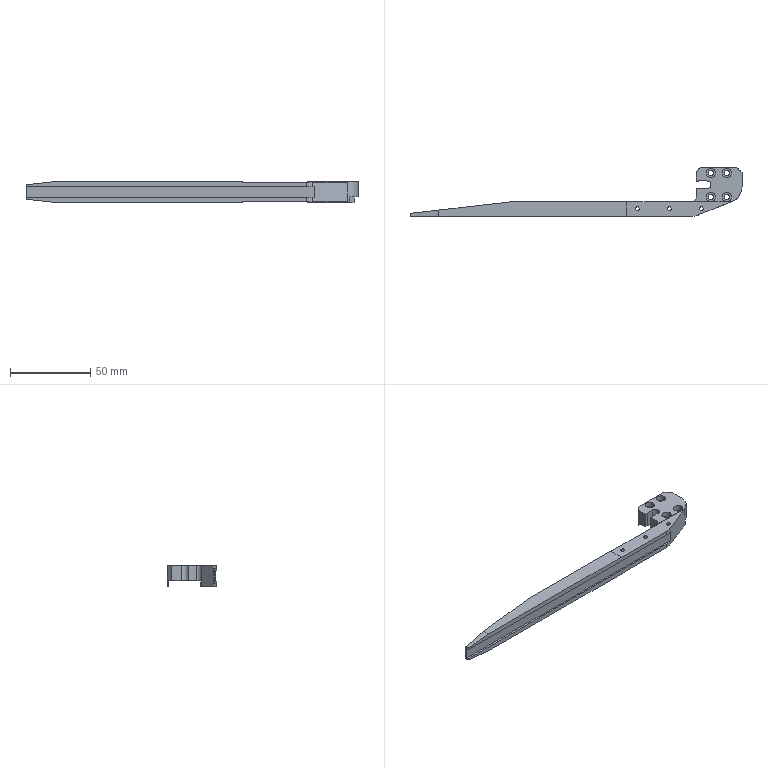NC program | NX | posted by the shop | part box 207.5 x 30.8 x 13 mm
Lines 3457 to 4469 of 6162:
N7 T17 M06
(D3-J  D=3. R=0. H=17 ce=0.00 di=0.01)
G00 G90 G54 X-72.98 Y-3.726 M03 S9000
G43 H17 Z20.
M08
Z-.139
G01 X-72.983 Y-3.731 Z-.207 F1600.
X-72.991 Y-3.747 Z-.269
X-73.002 Y-3.771 Z-.324
X-73.016 Y-3.804 Z-.372
X-73.032 Y-3.844 Z-.415
X-73.049 Y-3.889 Z-.453
X-73.065 Y-3.938 Z-.485
X-73.081 Y-3.991 Z-.512
X-73.094 Y-4.046 Z-.534
X-73.104 Y-4.102 Z-.552
X-73.109 Y-4.157 Z-.566
X-73.11 Y-4.212 Z-.576
X-73.105 Y-4.264 Z-.583
X-73.092 Y-4.312 Z-.587
X-73.071 Y-4.355 Z-.589
G03 X-72.25 Y-4.6 I.821 J1.255 F2000.
G01 X-71.604
X-71.564 Y-4.591 Z-.59
X-71.545 Y-4.565 Z-.594
X-71.544 Y-4.525 Z-.6
X-71.56 Y-4.475 Z-.608
X-71.59 Y-4.417 Z-.617
X-71.633 Y-4.355 Z-.629
X-71.687 Y-4.291 Z-.641
X-71.75 Y-4.229 Z-.654
X-71.82 Y-4.172 Z-.668
X-71.961 Y-4.088 Z-.695
X-72.116 Y-4.03 Z-.722
X-72.28 Y-3.999 Z-.75
X-72.451 Y-3.996 Z-.777
X-72.625 Y-4.021 Z-.803
X-72.72 Y-4.047 Z-.817
X-72.812 Y-4.08 Z-.831
X-72.897 Y-4.119 Z-.843
X-72.971 Y-4.16 Z-.854
X-73.032 Y-4.204 Z-.864
X-73.075 Y-4.247 Z-.872
X-73.099 Y-4.288 Z-.878
X-73.098 Y-4.325 Z-.882
X-73.071 Y-4.355 Z-.883
G03 X-72.25 Y-4.6 I.821 J1.255
G01 X-71.604
X-71.564 Y-4.591 Z-.884
X-71.545 Y-4.565 Z-.888
X-71.544 Y-4.525 Z-.894
X-71.56 Y-4.475 Z-.902
X-71.59 Y-4.417 Z-.912
X-71.633 Y-4.355 Z-.923
X-71.687 Y-4.291 Z-.935
X-71.75 Y-4.229 Z-.949
X-71.82 Y-4.172 Z-.963
X-71.961 Y-4.088 Z-.989
X-72.116 Y-4.03 Z-1.016
X-72.28 Y-3.999 Z-1.044
X-72.451 Y-3.996 Z-1.071
X-72.625 Y-4.021 Z-1.098
X-72.72 Y-4.047 Z-1.112
X-72.812 Y-4.08 Z-1.125
X-72.897 Y-4.119 Z-1.137
X-72.971 Y-4.16 Z-1.148
X-73.032 Y-4.204 Z-1.158
X-73.075 Y-4.247 Z-1.166
X-73.099 Y-4.288 Z-1.172
X-73.098 Y-4.325 Z-1.176
X-73.071 Y-4.355 Z-1.177
G03 X-72.25 Y-4.6 I.821 J1.255
G01 X-71.604
X-71.564 Y-4.591 Z-1.179
X-71.545 Y-4.565 Z-1.182
X-71.544 Y-4.525 Z-1.188
X-71.56 Y-4.475 Z-1.196
X-71.59 Y-4.417 Z-1.206
X-71.633 Y-4.355 Z-1.217
X-71.687 Y-4.291 Z-1.23
X-71.75 Y-4.229 Z-1.243
X-71.82 Y-4.172 Z-1.257
X-71.961 Y-4.088 Z-1.283
X-72.116 Y-4.03 Z-1.311
X-72.28 Y-3.999 Z-1.338
X-72.451 Y-3.996 Z-1.365
X-72.625 Y-4.021 Z-1.392
X-72.72 Y-4.047 Z-1.406
X-72.812 Y-4.08 Z-1.419
X-72.897 Y-4.119 Z-1.432
X-72.971 Y-4.16 Z-1.443
X-73.032 Y-4.204 Z-1.452
X-73.075 Y-4.247 Z-1.46
X-73.099 Y-4.288 Z-1.466
X-73.098 Y-4.325 Z-1.47
X-73.071 Y-4.355 Z-1.472
G03 X-72.25 Y-4.6 I.821 J1.255
G01 X-71.604
X-71.564 Y-4.591 Z-1.473
X-71.545 Y-4.565 Z-1.477
X-71.544 Y-4.525 Z-1.483
X-71.56 Y-4.475 Z-1.491
X-71.59 Y-4.417 Z-1.5
X-71.633 Y-4.355 Z-1.512
X-71.687 Y-4.291 Z-1.524
X-71.75 Y-4.229 Z-1.537
X-71.82 Y-4.172 Z-1.551
X-71.961 Y-4.088 Z-1.578
X-72.116 Y-4.03 Z-1.605
X-72.28 Y-3.999 Z-1.633
X-72.451 Y-3.996 Z-1.66
X-72.625 Y-4.021 Z-1.686
X-72.72 Y-4.047 Z-1.7
X-72.812 Y-4.08 Z-1.714
X-72.897 Y-4.119 Z-1.726
X-72.971 Y-4.16 Z-1.737
X-73.032 Y-4.204 Z-1.747
X-73.075 Y-4.247 Z-1.755
X-73.099 Y-4.288 Z-1.761
X-73.098 Y-4.325 Z-1.765
X-73.071 Y-4.355 Z-1.766
G03 X-72.25 Y-4.6 I.821 J1.255
G01 X-71.604
X-71.564 Y-4.591 Z-1.767
X-71.545 Y-4.565 Z-1.771
X-71.544 Y-4.525 Z-1.777
X-71.56 Y-4.475 Z-1.785
X-71.59 Y-4.417 Z-1.795
X-71.633 Y-4.355 Z-1.806
X-71.687 Y-4.291 Z-1.818
X-71.75 Y-4.229 Z-1.832
X-71.82 Y-4.172 Z-1.846
X-71.961 Y-4.088 Z-1.872
X-72.116 Y-4.03 Z-1.899
X-72.28 Y-3.999 Z-1.927
X-72.451 Y-3.996 Z-1.954
X-72.625 Y-4.021 Z-1.981
X-72.72 Y-4.047 Z-1.995
X-72.812 Y-4.08 Z-2.008
X-72.897 Y-4.119 Z-2.02
X-72.971 Y-4.16 Z-2.031
X-73.032 Y-4.204 Z-2.041
X-73.075 Y-4.247 Z-2.049
X-73.099 Y-4.288 Z-2.055
X-73.098 Y-4.325 Z-2.059
X-73.071 Y-4.355 Z-2.06
G03 X-72.25 Y-4.6 I.821 J1.255
G01 X-71.604
X-71.564 Y-4.591 Z-2.062
X-71.545 Y-4.565 Z-2.065
X-71.544 Y-4.525 Z-2.071
X-71.56 Y-4.475 Z-2.079
X-71.59 Y-4.417 Z-2.089
X-71.633 Y-4.355 Z-2.1
X-71.687 Y-4.291 Z-2.113
X-71.75 Y-4.229 Z-2.126
X-71.82 Y-4.172 Z-2.14
X-71.961 Y-4.088 Z-2.166
X-72.116 Y-4.03 Z-2.194
X-72.28 Y-3.999 Z-2.221
X-72.451 Y-3.996 Z-2.248
X-72.625 Y-4.021 Z-2.275
X-72.72 Y-4.047 Z-2.289
X-72.812 Y-4.08 Z-2.302
X-72.897 Y-4.119 Z-2.315
X-72.971 Y-4.16 Z-2.326
X-73.032 Y-4.204 Z-2.335
X-73.075 Y-4.247 Z-2.343
X-73.099 Y-4.288 Z-2.349
X-73.098 Y-4.325 Z-2.353
X-73.071 Y-4.355 Z-2.355
G03 X-72.25 Y-4.6 I.821 J1.255
G01 X-71.604
X-71.564 Y-4.591 Z-2.356
X-71.545 Y-4.565 Z-2.36
X-71.544 Y-4.525 Z-2.366
X-71.56 Y-4.475 Z-2.374
X-71.59 Y-4.417 Z-2.383
X-71.633 Y-4.355 Z-2.395
X-71.687 Y-4.291 Z-2.407
X-71.75 Y-4.229 Z-2.42
X-71.82 Y-4.172 Z-2.434
X-71.961 Y-4.088 Z-2.461
X-72.116 Y-4.03 Z-2.488
X-72.28 Y-3.999 Z-2.515
X-72.451 Y-3.996 Z-2.543
X-72.625 Y-4.021 Z-2.569
X-72.72 Y-4.047 Z-2.583
X-72.812 Y-4.08 Z-2.597
X-72.897 Y-4.119 Z-2.609
X-72.971 Y-4.16 Z-2.62
X-73.032 Y-4.204 Z-2.63
X-73.075 Y-4.247 Z-2.638
X-73.099 Y-4.288 Z-2.644
X-73.098 Y-4.325 Z-2.648
X-73.071 Y-4.355 Z-2.649
G03 X-72.25 Y-4.6 I.821 J1.255
G01 X-71.604
X-71.564 Y-4.591 Z-2.65
X-71.545 Y-4.565 Z-2.654
X-71.544 Y-4.525 Z-2.66
X-71.56 Y-4.475 Z-2.668
X-71.59 Y-4.417 Z-2.678
X-71.633 Y-4.355 Z-2.689
X-71.687 Y-4.291 Z-2.701
X-71.75 Y-4.229 Z-2.715
X-71.82 Y-4.172 Z-2.729
X-71.961 Y-4.088 Z-2.755
X-72.116 Y-4.03 Z-2.782
X-72.28 Y-3.999 Z-2.81
X-72.451 Y-3.996 Z-2.837
X-72.625 Y-4.021 Z-2.863
X-72.72 Y-4.047 Z-2.878
X-72.812 Y-4.08 Z-2.891
X-72.897 Y-4.119 Z-2.903
X-72.971 Y-4.16 Z-2.914
X-73.032 Y-4.204 Z-2.924
X-73.075 Y-4.247 Z-2.932
X-73.099 Y-4.288 Z-2.938
X-73.098 Y-4.325 Z-2.942
X-73.071 Y-4.355 Z-2.943
G03 X-72.25 Y-4.6 I.821 J1.255
G01 X-71.604
X-71.564 Y-4.591 Z-2.945
X-71.545 Y-4.565 Z-2.948
X-71.544 Y-4.525 Z-2.954
X-71.56 Y-4.475 Z-2.962
X-71.59 Y-4.417 Z-2.972
X-71.633 Y-4.355 Z-2.983
X-71.687 Y-4.291 Z-2.996
X-71.75 Y-4.229 Z-3.009
X-71.82 Y-4.172 Z-3.023
X-71.961 Y-4.088 Z-3.049
X-72.116 Y-4.03 Z-3.077
X-72.28 Y-3.999 Z-3.104
X-72.451 Y-3.996 Z-3.131
X-72.625 Y-4.021 Z-3.158
X-72.72 Y-4.047 Z-3.172
X-72.812 Y-4.08 Z-3.185
X-72.897 Y-4.119 Z-3.198
X-72.971 Y-4.16 Z-3.209
X-73.032 Y-4.204 Z-3.218
X-73.075 Y-4.247 Z-3.226
X-73.099 Y-4.288 Z-3.232
X-73.098 Y-4.325 Z-3.236
X-73.071 Y-4.355 Z-3.238
G03 X-72.25 Y-4.6 I.821 J1.255
G01 X-71.604
X-71.57 Y-4.584
X-71.552 Y-4.539 Z-3.241
X-71.548 Y-4.467 Z-3.245
X-71.556 Y-4.372 Z-3.251
X-71.576 Y-4.257 Z-3.257
X-71.606 Y-4.125 Z-3.265
X-71.693 Y-3.828 Z-3.284
X-71.758 Y-3.635 Z-3.296
X-71.877 Y-3.321 Z-3.317
X-72.079 Y-2.865 Z-3.35
X-72.312 Y-2.43 Z-3.385
X-72.573 Y-2.024 Z-3.419
X-72.863 Y-1.652 Z-3.452
X-72.986 Y-1.515 Z-3.465
X-73.111 Y-1.387 Z-3.477
X-73.233 Y-1.271 Z-3.488
X-73.35 Y-1.168 Z-3.499
X-73.458 Y-1.081 Z-3.508
X-73.554 Y-1.013 Z-3.516
X-73.635 Y-.966 Z-3.523
X-73.697 Y-.943 Z-3.528
X-73.736 Y-.945 Z-3.531
X-73.75 Y-.975 Z-3.532
Y-3.1
G03 X-72.25 Y-4.6 I1.5 J0.0
G01 X-70.125
X-70.096 Y-4.584 Z-3.533
X-70.091 Y-4.539 Z-3.535
X-70.107 Y-4.467 Z-3.539
X-70.143 Y-4.372 Z-3.545
X-70.197 Y-4.257 Z-3.552
X-70.267 Y-4.125 Z-3.56
X-70.448 Y-3.827 Z-3.578
X-70.575 Y-3.634 Z-3.591
X-70.798 Y-3.321 Z-3.612
X-71.168 Y-2.865 Z-3.645
X-71.572 Y-2.43 Z-3.679
X-72.006 Y-2.024 Z-3.713
X-72.462 Y-1.652 Z-3.746
X-72.777 Y-1.428 Z-3.767
X-72.971 Y-1.3 Z-3.78
X-73.271 Y-1.119 Z-3.798
X-73.404 Y-1.048 Z-3.806
X-73.52 Y-.994 Z-3.813
X-73.616 Y-.957 Z-3.819
X-73.688 Y-.941 Z-3.823
X-73.734 Y-.946 Z-3.825
X-73.75 Y-.975 Z-3.826
Y-3.1
G03 X-72.25 Y-4.6 I1.5 J0.0
G01 X-70.125
X-70.096 Y-4.584 Z-3.827
X-70.091 Y-4.539 Z-3.83
X-70.107 Y-4.467 Z-3.834
X-70.143 Y-4.372 Z-3.839
X-70.197 Y-4.257 Z-3.846
X-70.267 Y-4.125 Z-3.854
X-70.448 Y-3.827 Z-3.872
X-70.575 Y-3.634 Z-3.885
X-70.798 Y-3.321 Z-3.906
X-71.168 Y-2.865 Z-3.939
X-71.572 Y-2.43 Z-3.973
X-72.006 Y-2.024 Z-4.008
X-72.462 Y-1.652 Z-4.041
X-72.777 Y-1.428 Z-4.062
X-72.971 Y-1.3 Z-4.074
X-73.271 Y-1.119 Z-4.093
X-73.404 Y-1.048 Z-4.101
X-73.52 Y-.994 Z-4.107
X-73.616 Y-.957 Z-4.113
X-73.688 Y-.941 Z-4.117
X-73.734 Y-.946 Z-4.12
X-73.75 Y-.975
Y-3.1
G03 X-72.25 Y-4.6 I1.5 J0.0
G01 X-70.125
X-70.096 Y-4.584 Z-4.121
X-70.091 Y-4.539 Z-4.124
X-70.107 Y-4.467 Z-4.128
X-70.143 Y-4.372 Z-4.134
X-70.197 Y-4.257 Z-4.14
X-70.267 Y-4.125 Z-4.148
X-70.448 Y-3.827 Z-4.167
X-70.575 Y-3.634 Z-4.179
X-70.798 Y-3.321 Z-4.2
X-71.168 Y-2.865 Z-4.233
X-71.572 Y-2.43 Z-4.268
X-72.006 Y-2.024 Z-4.302
X-72.462 Y-1.652 Z-4.335
X-72.777 Y-1.428 Z-4.356
X-72.971 Y-1.3 Z-4.368
X-73.271 Y-1.119 Z-4.387
X-73.404 Y-1.048 Z-4.395
X-73.52 Y-.994 Z-4.402
X-73.616 Y-.957 Z-4.407
X-73.688 Y-.941 Z-4.411
X-73.734 Y-.946 Z-4.414
X-73.75 Y-.975 Z-4.415
Y-3.1
G03 X-72.25 Y-4.6 I1.5 J0.0
G01 X-70.125
X-70.096 Y-4.584 Z-4.416
X-70.091 Y-4.539 Z-4.418
X-70.107 Y-4.467 Z-4.422
X-70.143 Y-4.372 Z-4.428
X-70.197 Y-4.257 Z-4.435
X-70.267 Y-4.125 Z-4.443
X-70.448 Y-3.827 Z-4.461
X-70.575 Y-3.634 Z-4.474
X-70.798 Y-3.321 Z-4.494
X-71.168 Y-2.865 Z-4.528
X-71.572 Y-2.43 Z-4.562
X-72.006 Y-2.024 Z-4.596
X-72.462 Y-1.652 Z-4.629
X-72.777 Y-1.428 Z-4.65
X-72.971 Y-1.3 Z-4.663
X-73.271 Y-1.119 Z-4.681
X-73.404 Y-1.048 Z-4.689
X-73.52 Y-.994 Z-4.696
X-73.616 Y-.957 Z-4.702
X-73.688 Y-.941 Z-4.706
X-73.734 Y-.946 Z-4.708
X-73.75 Y-.975 Z-4.709
Y-3.1
G03 X-72.25 Y-4.6 I1.5 J0.0
G01 X-70.125
X-70.096 Y-4.584 Z-4.71
X-70.091 Y-4.539 Z-4.713
X-70.107 Y-4.467 Z-4.717
X-70.143 Y-4.372 Z-4.722
X-70.197 Y-4.257 Z-4.729
X-70.267 Y-4.125 Z-4.737
X-70.448 Y-3.827 Z-4.755
X-70.575 Y-3.634 Z-4.768
X-70.798 Y-3.321 Z-4.789
X-71.168 Y-2.865 Z-4.822
X-71.572 Y-2.43 Z-4.856
X-72.006 Y-2.024 Z-4.891
X-72.462 Y-1.652 Z-4.924
X-72.777 Y-1.428 Z-4.945
X-72.971 Y-1.3 Z-4.957
X-73.271 Y-1.119 Z-4.976
X-73.404 Y-1.048 Z-4.983
X-73.52 Y-.994 Z-4.99
X-73.616 Y-.957 Z-4.996
X-73.688 Y-.941 Z-5.
X-73.734 Y-.946 Z-5.003
X-73.75 Y-.975
Y-3.1
G03 X-72.25 Y-4.6 I1.5 J0.0
G01 X-70.125
X-70.096 Y-4.584 Z-5.004
X-70.091 Y-4.539 Z-5.007
X-70.107 Y-4.467 Z-5.011
X-70.143 Y-4.372 Z-5.017
X-70.197 Y-4.257 Z-5.023
X-70.267 Y-4.125 Z-5.031
X-70.448 Y-3.827 Z-5.05
X-70.575 Y-3.634 Z-5.062
X-70.798 Y-3.321 Z-5.083
X-71.168 Y-2.865 Z-5.116
X-71.572 Y-2.43 Z-5.151
X-72.006 Y-2.024 Z-5.185
X-72.462 Y-1.652 Z-5.218
X-72.777 Y-1.428 Z-5.239
X-72.971 Y-1.3 Z-5.251
X-73.271 Y-1.119 Z-5.27
X-73.404 Y-1.048 Z-5.278
X-73.52 Y-.994 Z-5.285
X-73.616 Y-.957 Z-5.29
X-73.688 Y-.941 Z-5.294
X-73.734 Y-.946 Z-5.297
X-73.75 Y-.975 Z-5.298
Y-3.1
G03 X-72.25 Y-4.6 I1.5 J0.0
G01 X-70.125
X-70.096 Y-4.584 Z-5.299
X-70.091 Y-4.539 Z-5.301
X-70.107 Y-4.467 Z-5.305
X-70.143 Y-4.372 Z-5.311
X-70.197 Y-4.257 Z-5.318
X-70.267 Y-4.125 Z-5.326
X-70.448 Y-3.827 Z-5.344
X-70.575 Y-3.634 Z-5.356
X-70.798 Y-3.321 Z-5.377
X-71.168 Y-2.865 Z-5.411
X-71.572 Y-2.43 Z-5.445
X-72.006 Y-2.024 Z-5.479
X-72.462 Y-1.652 Z-5.512
X-72.777 Y-1.428 Z-5.533
X-72.971 Y-1.3 Z-5.546
X-73.271 Y-1.119 Z-5.564
X-73.404 Y-1.048 Z-5.572
X-73.52 Y-.994 Z-5.579
X-73.616 Y-.957 Z-5.584
X-73.688 Y-.941 Z-5.589
X-73.734 Y-.946 Z-5.591
X-73.75 Y-.975 Z-5.592
Y-3.1
G03 X-72.25 Y-4.6 I1.5 J0.0
G01 X-70.125
X-70.096 Y-4.584 Z-5.593
X-70.091 Y-4.539 Z-5.596
X-70.107 Y-4.467 Z-5.6
X-70.143 Y-4.372 Z-5.605
X-70.197 Y-4.257 Z-5.612
X-70.267 Y-4.125 Z-5.62
X-70.448 Y-3.827 Z-5.638
X-70.575 Y-3.634 Z-5.651
X-70.798 Y-3.321 Z-5.672
X-71.168 Y-2.865 Z-5.705
X-71.572 Y-2.43 Z-5.739
X-72.006 Y-2.024 Z-5.774
X-72.462 Y-1.652 Z-5.807
X-72.777 Y-1.428 Z-5.828
X-72.971 Y-1.3 Z-5.84
X-73.271 Y-1.119 Z-5.859
X-73.404 Y-1.048 Z-5.866
X-73.52 Y-.994 Z-5.873
X-73.616 Y-.957 Z-5.879
X-73.688 Y-.941 Z-5.883
X-73.734 Y-.946 Z-5.885
X-73.75 Y-.975 Z-5.886
Y-3.1
G03 X-72.25 Y-4.6 I1.5 J0.0
G01 X-70.125
X-70.096 Y-4.584 Z-5.887
X-70.091 Y-4.539 Z-5.89
X-70.107 Y-4.467 Z-5.894
X-70.143 Y-4.372 Z-5.899
X-70.197 Y-4.257 Z-5.906
X-70.267 Y-4.125 Z-5.914
X-70.448 Y-3.827 Z-5.933
X-70.575 Y-3.634 Z-5.945
X-70.798 Y-3.321 Z-5.966
X-71.168 Y-2.865 Z-5.999
X-71.572 Y-2.43 Z-6.034
X-72.006 Y-2.024 Z-6.068
X-72.462 Y-1.652 Z-6.101
X-72.777 Y-1.428 Z-6.122
X-72.971 Y-1.3 Z-6.134
X-73.271 Y-1.119 Z-6.153
X-73.404 Y-1.048 Z-6.161
X-73.52 Y-.994 Z-6.168
X-73.616 Y-.957 Z-6.173
X-73.688 Y-.941 Z-6.177
X-73.734 Y-.946 Z-6.18
X-73.75 Y-.975 Z-6.181
Y-3.1
G03 X-72.25 Y-4.6 I1.5 J0.0
G01 X-70.125
X-70.096 Y-4.584 Z-6.182
X-70.091 Y-4.539 Z-6.184
X-70.107 Y-4.467 Z-6.188
X-70.143 Y-4.372 Z-6.194
X-70.197 Y-4.257 Z-6.201
X-70.267 Y-4.125 Z-6.209
X-70.448 Y-3.827 Z-6.227
X-70.575 Y-3.634 Z-6.239
X-70.798 Y-3.321 Z-6.26
X-71.168 Y-2.865 Z-6.294
X-71.572 Y-2.43 Z-6.328
X-72.006 Y-2.024 Z-6.362
X-72.462 Y-1.652 Z-6.395
X-72.777 Y-1.428 Z-6.416
X-72.971 Y-1.3 Z-6.429
X-73.271 Y-1.119 Z-6.447
X-73.404 Y-1.048 Z-6.455
X-73.52 Y-.994 Z-6.462
X-73.616 Y-.957 Z-6.467
X-73.688 Y-.941 Z-6.472
X-73.734 Y-.946 Z-6.474
X-73.75 Y-.975 Z-6.475
Y-3.1
G03 X-72.25 Y-4.6 I1.5 J0.0
G01 X-70.125
X-70.096 Y-4.584 Z-6.476
X-70.091 Y-4.539 Z-6.478
X-70.107 Y-4.467 Z-6.483
X-70.143 Y-4.372 Z-6.488
X-70.197 Y-4.257 Z-6.495
X-70.267 Y-4.125 Z-6.503
X-70.448 Y-3.827 Z-6.521
X-70.575 Y-3.634 Z-6.534
X-70.798 Y-3.321 Z-6.555
X-71.168 Y-2.865 Z-6.588
X-71.572 Y-2.43 Z-6.622
X-72.006 Y-2.024 Z-6.656
X-72.462 Y-1.652 Z-6.69
X-72.777 Y-1.428 Z-6.711
X-72.971 Y-1.3 Z-6.723
X-73.271 Y-1.119 Z-6.741
X-73.404 Y-1.048 Z-6.749
X-73.52 Y-.994 Z-6.756
X-73.616 Y-.957 Z-6.762
X-73.688 Y-.941 Z-6.766
X-73.734 Y-.946 Z-6.768
X-73.75 Y-.975 Z-6.769
Y-3.1
G03 X-72.25 Y-4.6 I1.5 J0.0
G01 X-70.125
X-70.096 Y-4.584 Z-6.77
X-70.091 Y-4.539 Z-6.773
X-70.107 Y-4.467 Z-6.777
X-70.143 Y-4.372 Z-6.782
X-70.197 Y-4.257 Z-6.789
X-70.267 Y-4.125 Z-6.797
X-70.448 Y-3.827 Z-6.816
X-70.575 Y-3.634 Z-6.828
X-70.798 Y-3.321 Z-6.849
X-71.168 Y-2.865 Z-6.882
X-71.572 Y-2.43 Z-6.916
X-72.006 Y-2.024 Z-6.951
X-72.462 Y-1.652 Z-6.984
X-72.777 Y-1.428 Z-7.005
X-72.971 Y-1.3 Z-7.017
X-73.271 Y-1.119 Z-7.036
X-73.404 Y-1.048 Z-7.044
X-73.52 Y-.994 Z-7.051
X-73.616 Y-.957 Z-7.056
X-73.688 Y-.941 Z-7.06
X-73.734 Y-.946 Z-7.063
X-73.75 Y-.975 Z-7.064
Y-3.1
G03 X-72.25 Y-4.6 I1.5 J0.0
G01 X-70.125
X-70.096 Y-4.584 Z-7.065
X-70.091 Y-4.539 Z-7.067
X-70.107 Y-4.467 Z-7.071
X-70.143 Y-4.372 Z-7.077
X-70.197 Y-4.257 Z-7.084
X-70.267 Y-4.125 Z-7.091
X-70.448 Y-3.827 Z-7.11
X-70.575 Y-3.634 Z-7.122
X-70.798 Y-3.321 Z-7.143
X-71.168 Y-2.865 Z-7.176
X-71.572 Y-2.43 Z-7.211
X-72.006 Y-2.024 Z-7.245
X-72.462 Y-1.652 Z-7.278
X-72.777 Y-1.428 Z-7.299
X-72.971 Y-1.3 Z-7.312
X-73.271 Y-1.119 Z-7.33
X-73.404 Y-1.048 Z-7.338
X-73.52 Y-.994 Z-7.345
X-73.616 Y-.957 Z-7.35
X-73.688 Y-.941 Z-7.354
X-73.734 Y-.946 Z-7.357
X-73.75 Y-.975 Z-7.358
Y-3.1
G03 X-72.25 Y-4.6 I1.5 J0.0
G01 X-70.125
X-70.096 Y-4.584 Z-7.359
X-70.091 Y-4.539 Z-7.361
X-70.107 Y-4.467 Z-7.366
X-70.143 Y-4.372 Z-7.371
X-70.197 Y-4.257 Z-7.378
X-70.267 Y-4.125 Z-7.386
X-70.448 Y-3.827 Z-7.404
X-70.575 Y-3.634 Z-7.417
X-70.798 Y-3.321 Z-7.438
X-71.168 Y-2.865 Z-7.471
X-71.572 Y-2.43 Z-7.505
X-72.006 Y-2.024 Z-7.539
X-72.462 Y-1.652 Z-7.573
X-72.777 Y-1.428 Z-7.594
X-72.971 Y-1.3 Z-7.606
X-73.271 Y-1.119 Z-7.624
X-73.404 Y-1.048 Z-7.632
X-73.52 Y-.994 Z-7.639
X-73.616 Y-.957 Z-7.645
X-73.688 Y-.941 Z-7.649
X-73.734 Y-.946 Z-7.651
X-73.75 Y-.975 Z-7.652
Y-3.1
G03 X-72.25 Y-4.6 I1.5 J0.0
G01 X-70.125
X-70.096 Y-4.584 Z-7.653
X-70.091 Y-4.539 Z-7.656
X-70.107 Y-4.467 Z-7.66
X-70.143 Y-4.372 Z-7.665
X-70.197 Y-4.257 Z-7.672
X-70.267 Y-4.125 Z-7.68
X-70.448 Y-3.827 Z-7.699
X-70.575 Y-3.634 Z-7.711
X-70.798 Y-3.321 Z-7.732
X-71.168 Y-2.865 Z-7.765
X-71.572 Y-2.43 Z-7.799
X-72.006 Y-2.024 Z-7.834
X-72.462 Y-1.652 Z-7.867
X-72.777 Y-1.428 Z-7.888
X-72.971 Y-1.3 Z-7.9
X-73.271 Y-1.119 Z-7.919
X-73.404 Y-1.048 Z-7.927
X-73.52 Y-.994 Z-7.933
X-73.616 Y-.957 Z-7.939
X-73.688 Y-.941 Z-7.943
X-73.734 Y-.946 Z-7.946
X-73.75 Y-.975 Z-7.947
Y-3.1
G03 X-72.25 Y-4.6 I1.5 J0.0
G01 X-70.125
X-70.096 Y-4.584
X-70.091 Y-4.539 Z-7.95
X-70.107 Y-4.467 Z-7.954
X-70.143 Y-4.372 Z-7.96
X-70.197 Y-4.257 Z-7.967
X-70.267 Y-4.125 Z-7.974
X-70.448 Y-3.827 Z-7.993
X-70.575 Y-3.634 Z-8.005
X-70.798 Y-3.321 Z-8.026
X-71.168 Y-2.865 Z-8.059
X-71.572 Y-2.43 Z-8.094
X-72.006 Y-2.024 Z-8.128
X-72.462 Y-1.652 Z-8.161
X-72.777 Y-1.428 Z-8.182
X-72.971 Y-1.3 Z-8.195
X-73.271 Y-1.119 Z-8.213
X-73.404 Y-1.048 Z-8.221
X-73.52 Y-.994 Z-8.228
X-73.616 Y-.957 Z-8.233
X-73.688 Y-.941 Z-8.237
X-73.734 Y-.946 Z-8.24
X-73.75 Y-.975 Z-8.241
Y-3.1
G03 X-72.25 Y-4.6 I1.5 J0.0
G01 X-70.125
X-70.096 Y-4.584 Z-8.242
X-70.091 Y-4.539 Z-8.244
X-70.107 Y-4.467 Z-8.248
X-70.143 Y-4.372 Z-8.254
X-70.197 Y-4.257 Z-8.261
X-70.267 Y-4.125 Z-8.269
X-70.448 Y-3.827 Z-8.287
X-70.575 Y-3.634 Z-8.3
X-70.798 Y-3.321 Z-8.321
X-71.168 Y-2.865 Z-8.354
X-71.572 Y-2.43 Z-8.388
X-72.006 Y-2.024 Z-8.422
X-72.462 Y-1.652 Z-8.456
X-72.777 Y-1.428 Z-8.476
X-72.971 Y-1.3 Z-8.489
X-73.271 Y-1.119 Z-8.507
X-73.404 Y-1.048 Z-8.515
X-73.52 Y-.994 Z-8.522
X-73.616 Y-.957 Z-8.528
X-73.688 Y-.941 Z-8.532
X-73.734 Y-.946 Z-8.534
X-73.75 Y-.975 Z-8.535
Y-3.1
G03 X-72.25 Y-4.6 I1.5 J0.0
G01 X-70.125
X-70.096 Y-4.584 Z-8.536
X-70.091 Y-4.539 Z-8.539
X-70.107 Y-4.467 Z-8.543
X-70.143 Y-4.372 Z-8.548
X-70.197 Y-4.257 Z-8.555
X-70.267 Y-4.125 Z-8.563
X-70.448 Y-3.827 Z-8.582
X-70.575 Y-3.634 Z-8.594
X-70.798 Y-3.321 Z-8.615
X-71.168 Y-2.865 Z-8.648
X-71.572 Y-2.43 Z-8.682
X-72.006 Y-2.024 Z-8.717
X-72.462 Y-1.652 Z-8.75
X-72.777 Y-1.428 Z-8.771
X-72.971 Y-1.3 Z-8.783
X-73.271 Y-1.119 Z-8.802
X-73.404 Y-1.048 Z-8.81
X-73.52 Y-.994 Z-8.816
X-73.616 Y-.957 Z-8.822
X-73.688 Y-.941 Z-8.826
X-73.734 Y-.946 Z-8.829
X-73.75 Y-.975 Z-8.83
Y-3.1
G03 X-72.25 Y-4.6 I1.5 J0.0
G01 X-70.125
X-70.096 Y-4.584
X-70.091 Y-4.539 Z-8.833
X-70.107 Y-4.467 Z-8.837
X-70.143 Y-4.372 Z-8.843
X-70.197 Y-4.257 Z-8.849
X-70.267 Y-4.125 Z-8.857
X-70.448 Y-3.827 Z-8.876
X-70.575 Y-3.634 Z-8.888
X-70.798 Y-3.321 Z-8.909
X-71.168 Y-2.865 Z-8.942
X-71.572 Y-2.43 Z-8.977
X-72.006 Y-2.024 Z-9.011
X-72.462 Y-1.652 Z-9.044
X-72.777 Y-1.428 Z-9.065
X-72.971 Y-1.3 Z-9.078
X-73.271 Y-1.119 Z-9.096
X-73.404 Y-1.048 Z-9.104
X-73.52 Y-.994 Z-9.111
X-73.616 Y-.957 Z-9.116
X-73.688 Y-.941 Z-9.12
X-73.734 Y-.946 Z-9.123
X-73.75 Y-.975 Z-9.124
Y-3.1
G03 X-72.25 Y-4.6 I1.5 J0.0
G01 X-70.125
X-70.096 Y-4.584 Z-9.125
X-70.091 Y-4.539 Z-9.127
X-70.107 Y-4.467 Z-9.131
X-70.143 Y-4.372 Z-9.137
X-70.197 Y-4.257 Z-9.144
X-70.267 Y-4.125 Z-9.152
X-70.448 Y-3.827 Z-9.17
X-70.575 Y-3.634 Z-9.183
X-70.798 Y-3.321 Z-9.204
X-71.168 Y-2.865 Z-9.237
X-71.572 Y-2.43 Z-9.271
X-72.006 Y-2.024 Z-9.305
X-72.462 Y-1.652 Z-9.338
X-72.777 Y-1.428 Z-9.359
X-72.971 Y-1.3 Z-9.372
X-73.271 Y-1.119 Z-9.39
X-73.404 Y-1.048 Z-9.398
X-73.52 Y-.994 Z-9.405
X-73.616 Y-.957 Z-9.411
X-73.688 Y-.941 Z-9.415
X-73.734 Y-.946 Z-9.417
X-73.75 Y-.975 Z-9.418
Y-3.1
G03 X-72.25 Y-4.6 I1.5 J0.0
G01 X-70.125
X-70.096 Y-4.584 Z-9.419
X-70.091 Y-4.539 Z-9.422
X-70.107 Y-4.467 Z-9.426
X-70.143 Y-4.372 Z-9.431
X-70.197 Y-4.257 Z-9.438
X-70.267 Y-4.125 Z-9.446
X-70.448 Y-3.827 Z-9.465
X-70.575 Y-3.634 Z-9.477
X-70.798 Y-3.321 Z-9.498
X-71.168 Y-2.865 Z-9.531
X-71.572 Y-2.43 Z-9.565
X-72.006 Y-2.024 Z-9.6
X-72.462 Y-1.652 Z-9.633
X-72.777 Y-1.428 Z-9.654
X-72.971 Y-1.3 Z-9.666
X-73.271 Y-1.119 Z-9.685
X-73.404 Y-1.048 Z-9.693
X-73.52 Y-.994 Z-9.699
X-73.616 Y-.957 Z-9.705
X-73.688 Y-.941 Z-9.709
X-73.734 Y-.946 Z-9.712
X-73.75 Y-.975 Z-9.713
Y-3.1
G03 X-72.25 Y-4.6 I1.5 J0.0
G01 X-70.125
X-70.096 Y-4.584
X-70.091 Y-4.539 Z-9.716
X-70.107 Y-4.467 Z-9.72
X-70.143 Y-4.372 Z-9.726
X-70.197 Y-4.257 Z-9.732
X-70.267 Y-4.125 Z-9.74
X-70.448 Y-3.827 Z-9.759
X-70.575 Y-3.634 Z-9.771
X-70.798 Y-3.321 Z-9.792
X-71.168 Y-2.865 Z-9.825
X-71.572 Y-2.43 Z-9.86
X-72.006 Y-2.024 Z-9.894
X-72.462 Y-1.652 Z-9.927
X-72.777 Y-1.428 Z-9.948
X-72.971 Y-1.3 Z-9.96
X-73.271 Y-1.119 Z-9.979
X-73.404 Y-1.048 Z-9.987
X-73.52 Y-.994 Z-9.994
X-73.616 Y-.957 Z-9.999
X-73.688 Y-.941 Z-10.003
X-73.734 Y-.946 Z-10.006
X-73.75 Y-.975 Z-10.007
Y-3.1
G03 X-72.25 Y-4.6 I1.5 J0.0
G01 X-70.125
X-70.096 Y-4.584 Z-10.008
X-70.091 Y-4.539 Z-10.01
X-70.107 Y-4.467 Z-10.014
X-70.143 Y-4.372 Z-10.02
X-70.197 Y-4.257 Z-10.027
X-70.267 Y-4.125 Z-10.035
X-70.448 Y-3.827 Z-10.053
X-70.575 Y-3.634 Z-10.066
X-70.798 Y-3.321 Z-10.087
X-71.168 Y-2.865 Z-10.12
X-71.572 Y-2.43 Z-10.154
X-72.006 Y-2.024 Z-10.188
X-72.462 Y-1.652 Z-10.221
X-72.777 Y-1.428 Z-10.242
X-72.971 Y-1.3 Z-10.255
X-73.271 Y-1.119 Z-10.273
X-73.404 Y-1.048 Z-10.281
X-73.52 Y-.994 Z-10.288
X-73.616 Y-.957 Z-10.294
X-73.688 Y-.941 Z-10.298
X-73.734 Y-.946 Z-10.3
X-73.75 Y-.975 Z-10.301
Y-3.1
G03 X-72.25 Y-4.6 I1.5 J0.0
G01 X-70.125
X-70.096 Y-4.584 Z-10.302
X-70.091 Y-4.539 Z-10.305
X-70.107 Y-4.467 Z-10.309
X-70.143 Y-4.372 Z-10.314
X-70.197 Y-4.257 Z-10.321
X-70.267 Y-4.125 Z-10.329
X-70.448 Y-3.827 Z-10.347
X-70.575 Y-3.634 Z-10.36
X-70.798 Y-3.321 Z-10.381
X-71.168 Y-2.865 Z-10.414
X-71.572 Y-2.43 Z-10.448
X-72.006 Y-2.024 Z-10.483
X-72.462 Y-1.652 Z-10.516
X-72.777 Y-1.428 Z-10.537
X-72.971 Y-1.3 Z-10.549
X-73.271 Y-1.119 Z-10.568
X-73.404 Y-1.048 Z-10.576
X-73.52 Y-.994 Z-10.582
X-73.616 Y-.957 Z-10.588
X-73.688 Y-.941 Z-10.592
X-73.734 Y-.946 Z-10.595
X-73.75 Y-.975
Y-3.1
G03 X-72.25 Y-4.6 I1.5 J0.0
G01 X-70.125
X-70.096 Y-4.584 Z-10.596
X-70.091 Y-4.539 Z-10.599
X-70.107 Y-4.467 Z-10.603
X-70.143 Y-4.372 Z-10.609
X-70.197 Y-4.257 Z-10.615
X-70.267 Y-4.125 Z-10.623
X-70.448 Y-3.827 Z-10.642
X-70.575 Y-3.634 Z-10.654
X-70.798 Y-3.321 Z-10.675
X-71.168 Y-2.865 Z-10.708
X-71.572 Y-2.43 Z-10.743
X-72.006 Y-2.024 Z-10.777
X-72.462 Y-1.652 Z-10.81
X-72.777 Y-1.428 Z-10.831
X-72.971 Y-1.3 Z-10.843
X-73.271 Y-1.119 Z-10.862
X-73.404 Y-1.048 Z-10.87
X-73.52 Y-.994 Z-10.877
X-73.616 Y-.957 Z-10.882
X-73.688 Y-.941 Z-10.886
X-73.734 Y-.946 Z-10.889
X-73.75 Y-.975 Z-10.89
Y-3.1
G03 X-72.25 Y-4.6 I1.5 J0.0
G01 X-70.125
X-70.096 Y-4.584 Z-10.891
X-70.091 Y-4.539 Z-10.893
X-70.107 Y-4.467 Z-10.897
X-70.143 Y-4.372 Z-10.903
X-70.197 Y-4.257 Z-10.91
X-70.267 Y-4.125 Z-10.918
X-70.448 Y-3.827 Z-10.936
X-70.575 Y-3.634 Z-10.949
X-70.798 Y-3.321 Z-10.969
X-71.168 Y-2.865 Z-11.003
X-71.572 Y-2.43 Z-11.037
X-72.006 Y-2.024 Z-11.071
X-72.462 Y-1.652 Z-11.104
X-72.777 Y-1.428 Z-11.125
X-72.971 Y-1.3 Z-11.138
X-73.271 Y-1.119 Z-11.156
X-73.404 Y-1.048 Z-11.164
X-73.52 Y-.994 Z-11.171
X-73.616 Y-.957 Z-11.177
X-73.688 Y-.941 Z-11.181
X-73.734 Y-.946 Z-11.183
X-73.75 Y-.975 Z-11.184
Y-3.1
G03 X-72.25 Y-4.6 I1.5 J0.0
G01 X-70.125
X-70.096 Y-4.584 Z-11.185
X-70.091 Y-4.539 Z-11.188
X-70.107 Y-4.467 Z-11.192
X-70.143 Y-4.372 Z-11.197
X-70.197 Y-4.257 Z-11.204
X-70.267 Y-4.125 Z-11.212
X-70.448 Y-3.827 Z-11.23
X-70.575 Y-3.634 Z-11.243
X-70.798 Y-3.321 Z-11.264
X-71.168 Y-2.865 Z-11.297
X-71.572 Y-2.43 Z-11.331
X-72.006 Y-2.024 Z-11.366
X-72.462 Y-1.652 Z-11.399
X-72.777 Y-1.428 Z-11.42
X-72.971 Y-1.3 Z-11.432
X-73.271 Y-1.119 Z-11.451
X-73.404 Y-1.048 Z-11.458
X-73.52 Y-.994 Z-11.465
X-73.616 Y-.957 Z-11.471
X-73.688 Y-.941 Z-11.475
X-73.734 Y-.946 Z-11.478
X-73.75 Y-.975
Y-3.1
G03 X-72.25 Y-4.6 I1.5 J0.0
G01 X-70.125
X-70.096 Y-4.584 Z-11.479
X-70.091 Y-4.539 Z-11.482
X-70.107 Y-4.467 Z-11.486
X-70.143 Y-4.372 Z-11.492
X-70.197 Y-4.257 Z-11.498
X-70.267 Y-4.125 Z-11.506
X-70.448 Y-3.827 Z-11.525
X-70.575 Y-3.634 Z-11.537
X-70.798 Y-3.321 Z-11.558
X-71.168 Y-2.865 Z-11.591
X-71.572 Y-2.43 Z-11.626
X-72.006 Y-2.024 Z-11.66
X-72.462 Y-1.652 Z-11.693
X-72.777 Y-1.428 Z-11.714
X-72.971 Y-1.3 Z-11.726
X-73.271 Y-1.119 Z-11.745
X-73.404 Y-1.048 Z-11.753
X-73.52 Y-.994 Z-11.76
X-73.616 Y-.957 Z-11.765
X-73.688 Y-.941 Z-11.769
X-73.734 Y-.946 Z-11.772
X-73.75 Y-.975 Z-11.773
Y-3.1
G03 X-72.25 Y-4.6 I1.5 J0.0
G01 X-70.125
X-70.096 Y-4.584 Z-11.774
X-70.091 Y-4.539 Z-11.776
X-70.107 Y-4.467 Z-11.78
X-70.143 Y-4.372 Z-11.786
X-70.197 Y-4.257 Z-11.793
X-70.267 Y-4.125 Z-11.801
X-70.448 Y-3.827 Z-11.819
X-70.575 Y-3.634 Z-11.831
X-70.798 Y-3.321 Z-11.852
X-71.168 Y-2.865 Z-11.886
X-71.572 Y-2.43 Z-11.92
X-72.006 Y-2.024 Z-11.954
X-72.462 Y-1.652 Z-11.987
X-72.777 Y-1.428 Z-12.008
X-72.971 Y-1.3 Z-12.021
X-73.271 Y-1.119 Z-12.039
X-73.404 Y-1.048 Z-12.047
X-73.52 Y-.994 Z-12.054
X-73.616 Y-.957 Z-12.059
X-73.688 Y-.941 Z-12.064
X-73.734 Y-.946 Z-12.066
X-73.75 Y-.975 Z-12.067
Y-3.1
G03 X-72.25 Y-4.6 I1.5 J0.0
G01 X-70.125
X-70.096 Y-4.584 Z-12.068
X-70.091 Y-4.539 Z-12.071
X-70.107 Y-4.467 Z-12.075
X-70.143 Y-4.372 Z-12.08
X-70.197 Y-4.257 Z-12.087
X-70.267 Y-4.125 Z-12.095
X-70.448 Y-3.827 Z-12.113
X-70.575 Y-3.634 Z-12.126
X-70.798 Y-3.321 Z-12.147
X-71.168 Y-2.865 Z-12.18
X-71.572 Y-2.43 Z-12.214
X-72.006 Y-2.024 Z-12.249
X-72.462 Y-1.652 Z-12.282
X-72.777 Y-1.428 Z-12.303